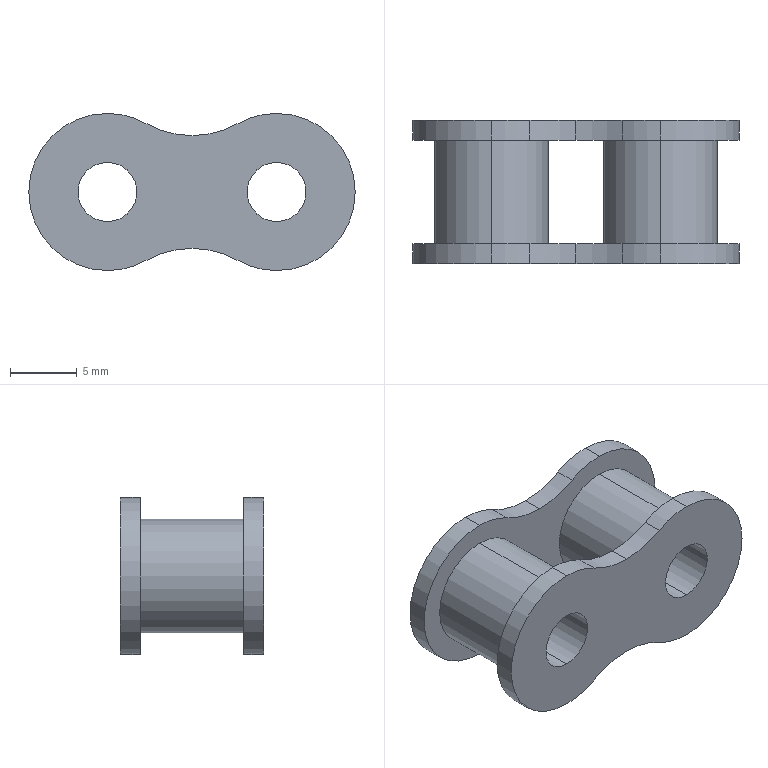Part | SolidWorks | features BaseBody 1 | 1 solid | 30 faces | box 24.5 x 10.75 x 11.8 mm | volume 1261 mm3 | cylinder 26 | plane 4 | commonest cylinder face diameters 11.8 x12 14.097 x6 4.44 x4 8.51 x4
STEP:
#1=CARTESIAN_POINT('',(-429.426,-311.093,-257.788));
#2=VERTEX_POINT('',#1);
#3=CARTESIAN_POINT('',(-429.426,-311.093,-253.348));
#4=VERTEX_POINT('',#3);
#5=CARTESIAN_POINT('',(-429.426,-311.093,-255.568));
#6=DIRECTION('',(0.,1.,0.));
#7=DIRECTION('',(0.,0.,-1.));
#8=AXIS2_PLACEMENT_3D('',#5,#6,#7);
#9=CIRCLE('',#8,2.22);
#10=EDGE_CURVE('',#2,#4,#9,.T.);
#11=ORIENTED_EDGE('',*,*,#10,.T.);
#12=CARTESIAN_POINT('',(-429.426,-321.843,-253.348));
#13=VERTEX_POINT('',#12);
#14=CARTESIAN_POINT('',(-429.426,-312.593,-253.348));
#15=DIRECTION('',(0.,-1.,0.));
#16=VECTOR('',#15,1000.);
#17=LINE('',#14,#16);
#18=EDGE_CURVE('',#4,#13,#17,.T.);
#19=ORIENTED_EDGE('',*,*,#18,.T.);
#20=CARTESIAN_POINT('',(-429.426,-321.843,-257.788));
#21=VERTEX_POINT('',#20);
#22=CARTESIAN_POINT('',(-429.426,-321.843,-255.568));
#23=DIRECTION('',(0.,1.,0.));
#24=DIRECTION('',(-1.,0.,0.));
#25=AXIS2_PLACEMENT_3D('',#22,#23,#24);
#26=CIRCLE('',#25,2.22);
#27=EDGE_CURVE('',#21,#13,#26,.T.);
#28=ORIENTED_EDGE('',*,*,#27,.F.);
#29=CARTESIAN_POINT('',(-429.426,-312.593,-257.788));
#30=DIRECTION('',(0.,-1.,0.));
#31=VECTOR('',#30,1000.);
#32=LINE('',#29,#31);
#33=EDGE_CURVE('',#2,#21,#32,.T.);
#34=ORIENTED_EDGE('',*,*,#33,.F.);
#35=EDGE_LOOP('',(#11,#19,#28,#34));
#36=FACE_OUTER_BOUND('',#35,.T.);
#37=CARTESIAN_POINT('',(-429.426,-312.593,-255.568));
#38=DIRECTION('',(0.,-1.,0.));
#39=DIRECTION('',(0.,0.,-1.));
#40=AXIS2_PLACEMENT_3D('',#37,#38,#39);
#41=CYLINDRICAL_SURFACE('',#40,2.22);
#42=ADVANCED_FACE('',(#36),#41,.F.);
#43=CARTESIAN_POINT('',(-429.426,-312.593,-251.313));
#44=VERTEX_POINT('',#43);
#45=CARTESIAN_POINT('',(-429.426,-312.593,-259.823));
#46=VERTEX_POINT('',#45);
#47=CARTESIAN_POINT('',(-429.426,-312.593,-255.568));
#48=DIRECTION('',(0.,1.,0.));
#49=DIRECTION('',(-1.,0.,0.));
#50=AXIS2_PLACEMENT_3D('',#47,#48,#49);
#51=CIRCLE('',#50,4.255);
#52=EDGE_CURVE('',#44,#46,#51,.T.);
#53=ORIENTED_EDGE('',*,*,#52,.F.);
#54=CARTESIAN_POINT('',(-429.426,-320.343,-251.313));
#55=VERTEX_POINT('',#54);
#56=CARTESIAN_POINT('',(-429.426,-312.593,-251.313));
#57=DIRECTION('',(0.,-1.,0.));
#58=VECTOR('',#57,1000.);
#59=LINE('',#56,#58);
#60=EDGE_CURVE('',#44,#55,#59,.T.);
#61=ORIENTED_EDGE('',*,*,#60,.T.);
#62=CARTESIAN_POINT('',(-429.426,-320.343,-259.823));
#63=VERTEX_POINT('',#62);
#64=CARTESIAN_POINT('',(-429.426,-320.343,-255.568));
#65=DIRECTION('',(0.,1.,0.));
#66=DIRECTION('',(0.,0.,-1.));
#67=AXIS2_PLACEMENT_3D('',#64,#65,#66);
#68=CIRCLE('',#67,4.255);
#69=EDGE_CURVE('',#55,#63,#68,.T.);
#70=ORIENTED_EDGE('',*,*,#69,.T.);
#71=CARTESIAN_POINT('',(-429.426,-312.593,-259.823));
#72=DIRECTION('',(0.,-1.,0.));
#73=VECTOR('',#72,1000.);
#74=LINE('',#71,#73);
#75=EDGE_CURVE('',#46,#63,#74,.T.);
#76=ORIENTED_EDGE('',*,*,#75,.F.);
#77=EDGE_LOOP('',(#53,#61,#70,#76));
#78=FACE_OUTER_BOUND('',#77,.T.);
#79=CARTESIAN_POINT('',(-429.426,-312.593,-255.568));
#80=DIRECTION('',(0.,-1.,0.));
#81=DIRECTION('',(0.,0.,-1.));
#82=AXIS2_PLACEMENT_3D('',#79,#80,#81);
#83=CYLINDRICAL_SURFACE('',#82,4.255);
#84=ADVANCED_FACE('',(#78),#83,.T.);
#85=CARTESIAN_POINT('',(-429.426,-311.093,-249.668));
#86=VERTEX_POINT('',#85);
#87=CARTESIAN_POINT('',(-429.426,-311.093,-261.468));
#88=VERTEX_POINT('',#87);
#89=CARTESIAN_POINT('',(-429.426,-311.093,-255.568));
#90=DIRECTION('',(0.,1.,0.));
#91=DIRECTION('',(-1.,0.,0.));
#92=AXIS2_PLACEMENT_3D('',#89,#90,#91);
#93=CIRCLE('',#92,5.9);
#94=EDGE_CURVE('',#86,#88,#93,.T.);
#95=ORIENTED_EDGE('',*,*,#94,.F.);
#96=CARTESIAN_POINT('',(-429.426,-312.593,-249.668));
#97=VERTEX_POINT('',#96);
#98=CARTESIAN_POINT('',(-429.426,-311.093,-249.668));
#99=DIRECTION('',(0.,-1.,0.));
#100=VECTOR('',#99,1000.);
#101=LINE('',#98,#100);
#102=EDGE_CURVE('',#86,#97,#101,.T.);
#103=ORIENTED_EDGE('',*,*,#102,.T.);
#104=CARTESIAN_POINT('',(-429.426,-312.593,-261.468));
#105=VERTEX_POINT('',#104);
#106=CARTESIAN_POINT('',(-429.426,-312.593,-255.568));
#107=DIRECTION('',(0.,1.,0.));
#108=DIRECTION('',(-1.,0.,0.));
#109=AXIS2_PLACEMENT_3D('',#106,#107,#108);
#110=CIRCLE('',#109,5.9);
#111=EDGE_CURVE('',#97,#105,#110,.T.);
#112=ORIENTED_EDGE('',*,*,#111,.T.);
#113=CARTESIAN_POINT('',(-429.426,-311.093,-261.468));
#114=DIRECTION('',(0.,-1.,0.));
#115=VECTOR('',#114,1000.);
#116=LINE('',#113,#115);
#117=EDGE_CURVE('',#88,#105,#116,.T.);
#118=ORIENTED_EDGE('',*,*,#117,.F.);
#119=EDGE_LOOP('',(#95,#103,#112,#118));
#120=FACE_OUTER_BOUND('',#119,.T.);
#121=CARTESIAN_POINT('',(-429.426,-311.093,-255.568));
#122=DIRECTION('',(0.,-1.,0.));
#123=DIRECTION('',(0.,0.,-1.));
#124=AXIS2_PLACEMENT_3D('',#121,#122,#123);
#125=CYLINDRICAL_SURFACE('',#124,5.9);
#126=ADVANCED_FACE('',(#120),#125,.T.);
#127=CARTESIAN_POINT('',(-432.319,-311.093,-260.71));
#128=VERTEX_POINT('',#127);
#129=CARTESIAN_POINT('',(-429.426,-311.093,-255.568));
#130=DIRECTION('',(0.,1.,0.));
#131=DIRECTION('',(-1.,0.,0.));
#132=AXIS2_PLACEMENT_3D('',#129,#130,#131);
#133=CIRCLE('',#132,5.9);
#134=EDGE_CURVE('',#88,#128,#133,.T.);
#135=ORIENTED_EDGE('',*,*,#134,.F.);
#136=ORIENTED_EDGE('',*,*,#117,.T.);
#137=CARTESIAN_POINT('',(-432.319,-312.593,-260.71));
#138=VERTEX_POINT('',#137);
#139=CARTESIAN_POINT('',(-429.426,-312.593,-255.568));
#140=DIRECTION('',(0.,1.,0.));
#141=DIRECTION('',(-1.,0.,0.));
#142=AXIS2_PLACEMENT_3D('',#139,#140,#141);
#143=CIRCLE('',#142,5.9);
#144=EDGE_CURVE('',#105,#138,#143,.T.);
#145=ORIENTED_EDGE('',*,*,#144,.T.);
#146=CARTESIAN_POINT('',(-432.319,-311.093,-260.71));
#147=DIRECTION('',(0.,-1.,0.));
#148=VECTOR('',#147,1000.);
#149=LINE('',#146,#148);
#150=EDGE_CURVE('',#128,#138,#149,.T.);
#151=ORIENTED_EDGE('',*,*,#150,.F.);
#152=EDGE_LOOP('',(#135,#136,#145,#151));
#153=FACE_OUTER_BOUND('',#152,.T.);
#154=CARTESIAN_POINT('',(-429.426,-311.093,-255.568));
#155=DIRECTION('',(0.,-1.,0.));
#156=DIRECTION('',(0.,0.,-1.));
#157=AXIS2_PLACEMENT_3D('',#154,#155,#156);
#158=CYLINDRICAL_SURFACE('',#157,5.9);
#159=ADVANCED_FACE('',(#153),#158,.T.);
#160=CARTESIAN_POINT('',(-435.776,-311.093,-251.332));
#161=VERTEX_POINT('',#160);
#162=CARTESIAN_POINT('',(-432.319,-311.093,-250.426));
#163=VERTEX_POINT('',#162);
#164=CARTESIAN_POINT('',(-435.776,-311.093,-244.284));
#165=DIRECTION('',(0.,-1.,0.));
#166=DIRECTION('',(-1.,0.,0.));
#167=AXIS2_PLACEMENT_3D('',#164,#165,#166);
#168=CIRCLE('',#167,7.048);
#169=EDGE_CURVE('',#161,#163,#168,.T.);
#170=ORIENTED_EDGE('',*,*,#169,.F.);
#171=CARTESIAN_POINT('',(-435.776,-312.593,-251.332));
#172=VERTEX_POINT('',#171);
#173=CARTESIAN_POINT('',(-435.776,-311.093,-251.332));
#174=DIRECTION('',(0.,-1.,0.));
#175=VECTOR('',#174,1000.);
#176=LINE('',#173,#175);
#177=EDGE_CURVE('',#161,#172,#176,.T.);
#178=ORIENTED_EDGE('',*,*,#177,.T.);
#179=CARTESIAN_POINT('',(-432.319,-312.593,-250.426));
#180=VERTEX_POINT('',#179);
#181=CARTESIAN_POINT('',(-435.776,-312.593,-244.284));
#182=DIRECTION('',(0.,-1.,0.));
#183=DIRECTION('',(-1.,0.,0.));
#184=AXIS2_PLACEMENT_3D('',#181,#182,#183);
#185=CIRCLE('',#184,7.048);
#186=EDGE_CURVE('',#172,#180,#185,.T.);
#187=ORIENTED_EDGE('',*,*,#186,.T.);
#188=CARTESIAN_POINT('',(-432.319,-311.093,-250.426));
#189=DIRECTION('',(0.,-1.,0.));
#190=VECTOR('',#189,1000.);
#191=LINE('',#188,#190);
#192=EDGE_CURVE('',#163,#180,#191,.T.);
#193=ORIENTED_EDGE('',*,*,#192,.F.);
#194=EDGE_LOOP('',(#170,#178,#187,#193));
#195=FACE_OUTER_BOUND('',#194,.T.);
#196=CARTESIAN_POINT('',(-435.776,-311.093,-244.284));
#197=DIRECTION('',(0.,-1.,0.));
#198=DIRECTION('',(0.,0.,-1.));
#199=AXIS2_PLACEMENT_3D('',#196,#197,#198);
#200=CYLINDRICAL_SURFACE('',#199,7.048);
#201=ADVANCED_FACE('',(#195),#200,.F.);
#202=CARTESIAN_POINT('',(-442.126,-311.093,-249.668));
#203=VERTEX_POINT('',#202);
#204=CARTESIAN_POINT('',(-439.232,-311.093,-250.426));
#205=VERTEX_POINT('',#204);
#206=CARTESIAN_POINT('',(-442.126,-311.093,-255.568));
#207=DIRECTION('',(0.,1.,0.));
#208=DIRECTION('',(-1.,0.,0.));
#209=AXIS2_PLACEMENT_3D('',#206,#207,#208);
#210=CIRCLE('',#209,5.9);
#211=EDGE_CURVE('',#203,#205,#210,.T.);
#212=ORIENTED_EDGE('',*,*,#211,.F.);
#213=CARTESIAN_POINT('',(-442.126,-312.593,-249.668));
#214=VERTEX_POINT('',#213);
#215=CARTESIAN_POINT('',(-442.126,-311.093,-249.668));
#216=DIRECTION('',(0.,-1.,0.));
#217=VECTOR('',#216,1000.);
#218=LINE('',#215,#217);
#219=EDGE_CURVE('',#203,#214,#218,.T.);
#220=ORIENTED_EDGE('',*,*,#219,.T.);
#221=CARTESIAN_POINT('',(-439.232,-312.593,-250.426));
#222=VERTEX_POINT('',#221);
#223=CARTESIAN_POINT('',(-442.126,-312.593,-255.568));
#224=DIRECTION('',(0.,1.,0.));
#225=DIRECTION('',(-1.,0.,0.));
#226=AXIS2_PLACEMENT_3D('',#223,#224,#225);
#227=CIRCLE('',#226,5.9);
#228=EDGE_CURVE('',#214,#222,#227,.T.);
#229=ORIENTED_EDGE('',*,*,#228,.T.);
#230=CARTESIAN_POINT('',(-439.232,-311.093,-250.426));
#231=DIRECTION('',(0.,-1.,0.));
#232=VECTOR('',#231,1000.);
#233=LINE('',#230,#232);
#234=EDGE_CURVE('',#205,#222,#233,.T.);
#235=ORIENTED_EDGE('',*,*,#234,.F.);
#236=EDGE_LOOP('',(#212,#220,#229,#235));
#237=FACE_OUTER_BOUND('',#236,.T.);
#238=CARTESIAN_POINT('',(-442.126,-311.093,-255.568));
#239=DIRECTION('',(0.,-1.,0.));
#240=DIRECTION('',(0.,0.,-1.));
#241=AXIS2_PLACEMENT_3D('',#238,#239,#240);
#242=CYLINDRICAL_SURFACE('',#241,5.9);
#243=ADVANCED_FACE('',(#237),#242,.T.);
#244=ORIENTED_EDGE('',*,*,#219,.F.);
#245=CARTESIAN_POINT('',(-442.126,-311.093,-261.468));
#246=VERTEX_POINT('',#245);
#247=CARTESIAN_POINT('',(-442.126,-311.093,-255.568));
#248=DIRECTION('',(0.,1.,0.));
#249=DIRECTION('',(-1.,0.,0.));
#250=AXIS2_PLACEMENT_3D('',#247,#248,#249);
#251=CIRCLE('',#250,5.9);
#252=EDGE_CURVE('',#246,#203,#251,.T.);
#253=ORIENTED_EDGE('',*,*,#252,.F.);
#254=CARTESIAN_POINT('',(-442.126,-312.593,-261.468));
#255=VERTEX_POINT('',#254);
#256=CARTESIAN_POINT('',(-442.126,-311.093,-261.468));
#257=DIRECTION('',(0.,-1.,0.));
#258=VECTOR('',#257,1000.);
#259=LINE('',#256,#258);
#260=EDGE_CURVE('',#246,#255,#259,.T.);
#261=ORIENTED_EDGE('',*,*,#260,.T.);
#262=CARTESIAN_POINT('',(-442.126,-312.593,-255.568));
#263=DIRECTION('',(0.,1.,0.));
#264=DIRECTION('',(-1.,0.,0.));
#265=AXIS2_PLACEMENT_3D('',#262,#263,#264);
#266=CIRCLE('',#265,5.9);
#267=EDGE_CURVE('',#255,#214,#266,.T.);
#268=ORIENTED_EDGE('',*,*,#267,.T.);
#269=EDGE_LOOP('',(#244,#253,#261,#268));
#270=FACE_OUTER_BOUND('',#269,.T.);
#271=CARTESIAN_POINT('',(-442.126,-311.093,-255.568));
#272=DIRECTION('',(0.,-1.,0.));
#273=DIRECTION('',(0.,0.,-1.));
#274=AXIS2_PLACEMENT_3D('',#271,#272,#273);
#275=CYLINDRICAL_SURFACE('',#274,5.9);
#276=ADVANCED_FACE('',(#270),#275,.T.);
#277=CARTESIAN_POINT('',(-429.426,-320.343,-249.668));
#278=VERTEX_POINT('',#277);
#279=CARTESIAN_POINT('',(-429.426,-320.343,-261.468));
#280=VERTEX_POINT('',#279);
#281=CARTESIAN_POINT('',(-429.426,-320.343,-255.568));
#282=DIRECTION('',(0.,1.,0.));
#283=DIRECTION('',(-1.,0.,0.));
#284=AXIS2_PLACEMENT_3D('',#281,#282,#283);
#285=CIRCLE('',#284,5.9);
#286=EDGE_CURVE('',#278,#280,#285,.T.);
#287=ORIENTED_EDGE('',*,*,#286,.F.);
#288=CARTESIAN_POINT('',(-429.426,-321.843,-249.668));
#289=VERTEX_POINT('',#288);
#290=CARTESIAN_POINT('',(-429.426,-320.343,-249.668));
#291=DIRECTION('',(0.,-1.,0.));
#292=VECTOR('',#291,1000.);
#293=LINE('',#290,#292);
#294=EDGE_CURVE('',#278,#289,#293,.T.);
#295=ORIENTED_EDGE('',*,*,#294,.T.);
#296=CARTESIAN_POINT('',(-429.426,-321.843,-261.468));
#297=VERTEX_POINT('',#296);
#298=CARTESIAN_POINT('',(-429.426,-321.843,-255.568));
#299=DIRECTION('',(0.,1.,0.));
#300=DIRECTION('',(-1.,0.,0.));
#301=AXIS2_PLACEMENT_3D('',#298,#299,#300);
#302=CIRCLE('',#301,5.9);
#303=EDGE_CURVE('',#289,#297,#302,.T.);
#304=ORIENTED_EDGE('',*,*,#303,.T.);
#305=CARTESIAN_POINT('',(-429.426,-320.343,-261.468));
#306=DIRECTION('',(0.,-1.,0.));
#307=VECTOR('',#306,1000.);
#308=LINE('',#305,#307);
#309=EDGE_CURVE('',#280,#297,#308,.T.);
#310=ORIENTED_EDGE('',*,*,#309,.F.);
#311=EDGE_LOOP('',(#287,#295,#304,#310));
#312=FACE_OUTER_BOUND('',#311,.T.);
#313=CARTESIAN_POINT('',(-429.426,-320.343,-255.568));
#314=DIRECTION('',(0.,-1.,0.));
#315=DIRECTION('',(0.,0.,-1.));
#316=AXIS2_PLACEMENT_3D('',#313,#314,#315);
#317=CYLINDRICAL_SURFACE('',#316,5.9);
#318=ADVANCED_FACE('',(#312),#317,.T.);
#319=CARTESIAN_POINT('',(-432.319,-320.343,-260.71));
#320=VERTEX_POINT('',#319);
#321=CARTESIAN_POINT('',(-429.426,-320.343,-255.568));
#322=DIRECTION('',(0.,1.,0.));
#323=DIRECTION('',(-1.,0.,0.));
#324=AXIS2_PLACEMENT_3D('',#321,#322,#323);
#325=CIRCLE('',#324,5.9);
#326=EDGE_CURVE('',#280,#320,#325,.T.);
#327=ORIENTED_EDGE('',*,*,#326,.F.);
#328=ORIENTED_EDGE('',*,*,#309,.T.);
#329=CARTESIAN_POINT('',(-432.319,-321.843,-260.71));
#330=VERTEX_POINT('',#329);
#331=CARTESIAN_POINT('',(-429.426,-321.843,-255.568));
#332=DIRECTION('',(0.,1.,0.));
#333=DIRECTION('',(-1.,0.,0.));
#334=AXIS2_PLACEMENT_3D('',#331,#332,#333);
#335=CIRCLE('',#334,5.9);
#336=EDGE_CURVE('',#297,#330,#335,.T.);
#337=ORIENTED_EDGE('',*,*,#336,.T.);
#338=CARTESIAN_POINT('',(-432.319,-320.343,-260.71));
#339=DIRECTION('',(0.,-1.,0.));
#340=VECTOR('',#339,1000.);
#341=LINE('',#338,#340);
#342=EDGE_CURVE('',#320,#330,#341,.T.);
#343=ORIENTED_EDGE('',*,*,#342,.F.);
#344=EDGE_LOOP('',(#327,#328,#337,#343));
#345=FACE_OUTER_BOUND('',#344,.T.);
#346=CARTESIAN_POINT('',(-429.426,-320.343,-255.568));
#347=DIRECTION('',(0.,-1.,0.));
#348=DIRECTION('',(0.,0.,-1.));
#349=AXIS2_PLACEMENT_3D('',#346,#347,#348);
#350=CYLINDRICAL_SURFACE('',#349,5.9);
#351=ADVANCED_FACE('',(#345),#350,.T.);
#352=CARTESIAN_POINT('',(-435.776,-320.343,-251.332));
#353=VERTEX_POINT('',#352);
#354=CARTESIAN_POINT('',(-432.319,-320.343,-250.426));
#355=VERTEX_POINT('',#354);
#356=CARTESIAN_POINT('',(-435.776,-320.343,-244.284));
#357=DIRECTION('',(0.,-1.,0.));
#358=DIRECTION('',(-1.,0.,0.));
#359=AXIS2_PLACEMENT_3D('',#356,#357,#358);
#360=CIRCLE('',#359,7.048);
#361=EDGE_CURVE('',#353,#355,#360,.T.);
#362=ORIENTED_EDGE('',*,*,#361,.F.);
#363=CARTESIAN_POINT('',(-435.776,-321.843,-251.332));
#364=VERTEX_POINT('',#363);
#365=CARTESIAN_POINT('',(-435.776,-320.343,-251.332));
#366=DIRECTION('',(0.,-1.,0.));
#367=VECTOR('',#366,1000.);
#368=LINE('',#365,#367);
#369=EDGE_CURVE('',#353,#364,#368,.T.);
#370=ORIENTED_EDGE('',*,*,#369,.T.);
#371=CARTESIAN_POINT('',(-432.319,-321.843,-250.426));
#372=VERTEX_POINT('',#371);
#373=CARTESIAN_POINT('',(-435.776,-321.843,-244.284));
#374=DIRECTION('',(0.,-1.,0.));
#375=DIRECTION('',(-1.,0.,0.));
#376=AXIS2_PLACEMENT_3D('',#373,#374,#375);
#377=CIRCLE('',#376,7.048);
#378=EDGE_CURVE('',#364,#372,#377,.T.);
#379=ORIENTED_EDGE('',*,*,#378,.T.);
#380=CARTESIAN_POINT('',(-432.319,-320.343,-250.426));
#381=DIRECTION('',(0.,-1.,0.));
#382=VECTOR('',#381,1000.);
#383=LINE('',#380,#382);
#384=EDGE_CURVE('',#355,#372,#383,.T.);
#385=ORIENTED_EDGE('',*,*,#384,.F.);
#386=EDGE_LOOP('',(#362,#370,#379,#385));
#387=FACE_OUTER_BOUND('',#386,.T.);
#388=CARTESIAN_POINT('',(-435.776,-320.343,-244.284));
#389=DIRECTION('',(0.,-1.,0.));
#390=DIRECTION('',(0.,0.,-1.));
#391=AXIS2_PLACEMENT_3D('',#388,#389,#390);
#392=CYLINDRICAL_SURFACE('',#391,7.048);
#393=ADVANCED_FACE('',(#387),#392,.F.);
#394=CARTESIAN_POINT('',(-442.126,-320.343,-249.668));
#395=VERTEX_POINT('',#394);
#396=CARTESIAN_POINT('',(-439.232,-320.343,-250.426));
#397=VERTEX_POINT('',#396);
#398=CARTESIAN_POINT('',(-442.126,-320.343,-255.568));
#399=DIRECTION('',(0.,1.,0.));
#400=DIRECTION('',(-1.,0.,0.));
#401=AXIS2_PLACEMENT_3D('',#398,#399,#400);
#402=CIRCLE('',#401,5.9);
#403=EDGE_CURVE('',#395,#397,#402,.T.);
#404=ORIENTED_EDGE('',*,*,#403,.F.);
#405=CARTESIAN_POINT('',(-442.126,-321.843,-249.668));
#406=VERTEX_POINT('',#405);
#407=CARTESIAN_POINT('',(-442.126,-320.343,-249.668));
#408=DIRECTION('',(0.,-1.,0.));
#409=VECTOR('',#408,1000.);
#410=LINE('',#407,#409);
#411=EDGE_CURVE('',#395,#406,#410,.T.);
#412=ORIENTED_EDGE('',*,*,#411,.T.);
#413=CARTESIAN_POINT('',(-439.232,-321.843,-250.426));
#414=VERTEX_POINT('',#413);
#415=CARTESIAN_POINT('',(-442.126,-321.843,-255.568));
#416=DIRECTION('',(0.,1.,0.));
#417=DIRECTION('',(-1.,0.,0.));
#418=AXIS2_PLACEMENT_3D('',#415,#416,#417);
#419=CIRCLE('',#418,5.9);
#420=EDGE_CURVE('',#406,#414,#419,.T.);
#421=ORIENTED_EDGE('',*,*,#420,.T.);
#422=CARTESIAN_POINT('',(-439.232,-320.343,-250.426));
#423=DIRECTION('',(0.,-1.,0.));
#424=VECTOR('',#423,1000.);
#425=LINE('',#422,#424);
#426=EDGE_CURVE('',#397,#414,#425,.T.);
#427=ORIENTED_EDGE('',*,*,#426,.F.);
#428=EDGE_LOOP('',(#404,#412,#421,#427));
#429=FACE_OUTER_BOUND('',#428,.T.);
#430=CARTESIAN_POINT('',(-442.126,-320.343,-255.568));
#431=DIRECTION('',(0.,-1.,0.));
#432=DIRECTION('',(0.,0.,-1.));
#433=AXIS2_PLACEMENT_3D('',#430,#431,#432);
#434=CYLINDRICAL_SURFACE('',#433,5.9);
#435=ADVANCED_FACE('',(#429),#434,.T.);
#436=ORIENTED_EDGE('',*,*,#411,.F.);
#437=CARTESIAN_POINT('',(-442.126,-320.343,-261.468));
#438=VERTEX_POINT('',#437);
#439=CARTESIAN_POINT('',(-442.126,-320.343,-255.568));
#440=DIRECTION('',(0.,1.,0.));
#441=DIRECTION('',(-1.,0.,0.));
#442=AXIS2_PLACEMENT_3D('',#439,#440,#441);
#443=CIRCLE('',#442,5.9);
#444=EDGE_CURVE('',#438,#395,#443,.T.);
#445=ORIENTED_EDGE('',*,*,#444,.F.);
#446=CARTESIAN_POINT('',(-442.126,-321.843,-261.468));
#447=VERTEX_POINT('',#446);
#448=CARTESIAN_POINT('',(-442.126,-320.343,-261.468));
#449=DIRECTION('',(0.,-1.,0.));
#450=VECTOR('',#449,1000.);
#451=LINE('',#448,#450);
#452=EDGE_CURVE('',#438,#447,#451,.T.);
#453=ORIENTED_EDGE('',*,*,#452,.T.);
#454=CARTESIAN_POINT('',(-442.126,-321.843,-255.568));
#455=DIRECTION('',(0.,1.,0.));
#456=DIRECTION('',(-1.,0.,0.));
#457=AXIS2_PLACEMENT_3D('',#454,#455,#456);
#458=CIRCLE('',#457,5.9);
#459=EDGE_CURVE('',#447,#406,#458,.T.);
#460=ORIENTED_EDGE('',*,*,#459,.T.);
#461=EDGE_LOOP('',(#436,#445,#453,#460));
#462=FACE_OUTER_BOUND('',#461,.T.);
#463=CARTESIAN_POINT('',(-442.126,-320.343,-255.568));
#464=DIRECTION('',(0.,-1.,0.));
#465=DIRECTION('',(0.,0.,-1.));
#466=AXIS2_PLACEMENT_3D('',#463,#464,#465);
#467=CYLINDRICAL_SURFACE('',#466,5.9);
#468=ADVANCED_FACE('',(#462),#467,.T.);
#469=CARTESIAN_POINT('',(-442.126,-311.093,-257.788));
#470=VERTEX_POINT('',#469);
#471=CARTESIAN_POINT('',(-442.126,-311.093,-253.348));
#472=VERTEX_POINT('',#471);
#473=CARTESIAN_POINT('',(-442.126,-311.093,-255.568));
#474=DIRECTION('',(0.,1.,0.));
#475=DIRECTION('',(0.,0.,-1.));
#476=AXIS2_PLACEMENT_3D('',#473,#474,#475);
#477=CIRCLE('',#476,2.22);
#478=EDGE_CURVE('',#470,#472,#477,.T.);
#479=ORIENTED_EDGE('',*,*,#478,.T.);
#480=CARTESIAN_POINT('',(-442.126,-321.843,-253.348));
#481=VERTEX_POINT('',#480);
#482=CARTESIAN_POINT('',(-442.126,-312.593,-253.348));
#483=DIRECTION('',(0.,-1.,0.));
#484=VECTOR('',#483,1000.);
#485=LINE('',#482,#484);
#486=EDGE_CURVE('',#472,#481,#485,.T.);
#487=ORIENTED_EDGE('',*,*,#486,.T.);
#488=CARTESIAN_POINT('',(-442.126,-321.843,-257.788));
#489=VERTEX_POINT('',#488);
#490=CARTESIAN_POINT('',(-442.126,-321.843,-255.568));
#491=DIRECTION('',(0.,1.,0.));
#492=DIRECTION('',(-1.,0.,0.));
#493=AXIS2_PLACEMENT_3D('',#490,#491,#492);
#494=CIRCLE('',#493,2.22);
#495=EDGE_CURVE('',#489,#481,#494,.T.);
#496=ORIENTED_EDGE('',*,*,#495,.F.);
#497=CARTESIAN_POINT('',(-442.126,-312.593,-257.788));
#498=DIRECTION('',(0.,-1.,0.));
#499=VECTOR('',#498,1000.);
#500=LINE('',#497,#499);
#501=EDGE_CURVE('',#470,#489,#500,.T.);
#502=ORIENTED_EDGE('',*,*,#501,.F.);
#503=EDGE_LOOP('',(#479,#487,#496,#502));
#504=FACE_OUTER_BOUND('',#503,.T.);
#505=CARTESIAN_POINT('',(-442.126,-312.593,-255.568));
#506=DIRECTION('',(0.,-1.,0.));
#507=DIRECTION('',(0.,0.,-1.));
#508=AXIS2_PLACEMENT_3D('',#505,#506,#507);
#509=CYLINDRICAL_SURFACE('',#508,2.22);
#510=ADVANCED_FACE('',(#504),#509,.F.);
#511=CARTESIAN_POINT('',(-442.126,-312.593,-259.823));
#512=VERTEX_POINT('',#511);
#513=CARTESIAN_POINT('',(-442.126,-312.593,-251.313));
#514=VERTEX_POINT('',#513);
#515=CARTESIAN_POINT('',(-442.126,-312.593,-255.568));
#516=DIRECTION('',(0.,-1.,0.));
#517=DIRECTION('',(0.,0.,-1.));
#518=AXIS2_PLACEMENT_3D('',#515,#516,#517);
#519=CIRCLE('',#518,4.255);
#520=EDGE_CURVE('',#512,#514,#519,.T.);
#521=ORIENTED_EDGE('',*,*,#520,.T.);
#522=CARTESIAN_POINT('',(-442.126,-320.343,-251.313));
#523=VERTEX_POINT('',#522);
#524=CARTESIAN_POINT('',(-442.126,-312.593,-251.313));
#525=DIRECTION('',(0.,-1.,0.));
#526=VECTOR('',#525,1000.);
#527=LINE('',#524,#526);
#528=EDGE_CURVE('',#514,#523,#527,.T.);
#529=ORIENTED_EDGE('',*,*,#528,.T.);
#530=CARTESIAN_POINT('',(-442.126,-320.343,-259.823));
#531=VERTEX_POINT('',#530);
#532=CARTESIAN_POINT('',(-442.126,-320.343,-255.568));
#533=DIRECTION('',(0.,1.,0.));
#534=DIRECTION('',(-1.,0.,0.));
#535=AXIS2_PLACEMENT_3D('',#532,#533,#534);
#536=CIRCLE('',#535,4.255);
#537=EDGE_CURVE('',#523,#531,#536,.T.);
#538=ORIENTED_EDGE('',*,*,#537,.T.);
#539=CARTESIAN_POINT('',(-442.126,-312.593,-259.823));
#540=DIRECTION('',(0.,-1.,0.));
#541=VECTOR('',#540,1000.);
#542=LINE('',#539,#541);
#543=EDGE_CURVE('',#512,#531,#542,.T.);
#544=ORIENTED_EDGE('',*,*,#543,.F.);
#545=EDGE_LOOP('',(#521,#529,#538,#544));
#546=FACE_OUTER_BOUND('',#545,.T.);
#547=CARTESIAN_POINT('',(-442.126,-312.593,-255.568));
#548=DIRECTION('',(0.,-1.,0.));
#549=DIRECTION('',(0.,0.,-1.));
#550=AXIS2_PLACEMENT_3D('',#547,#548,#549);
#551=CYLINDRICAL_SURFACE('',#550,4.255);
#552=ADVANCED_FACE('',(#546),#551,.T.);
#553=ORIENTED_EDGE('',*,*,#528,.F.);
#554=CARTESIAN_POINT('',(-442.126,-312.593,-255.568));
#555=DIRECTION('',(0.,-1.,0.));
#556=DIRECTION('',(0.,0.,-1.));
#557=AXIS2_PLACEMENT_3D('',#554,#555,#556);
#558=CIRCLE('',#557,4.255);
#559=EDGE_CURVE('',#514,#512,#558,.T.);
#560=ORIENTED_EDGE('',*,*,#559,.T.);
#561=ORIENTED_EDGE('',*,*,#543,.T.);
#562=CARTESIAN_POINT('',(-442.126,-320.343,-255.568));
#563=DIRECTION('',(0.,1.,0.));
#564=DIRECTION('',(-1.,0.,0.));
#565=AXIS2_PLACEMENT_3D('',#562,#563,#564);
#566=CIRCLE('',#565,4.255);
#567=EDGE_CURVE('',#531,#523,#566,.T.);
#568=ORIENTED_EDGE('',*,*,#567,.T.);
#569=EDGE_LOOP('',(#553,#560,#561,#568));
#570=FACE_OUTER_BOUND('',#569,.T.);
#571=CARTESIAN_POINT('',(-442.126,-312.593,-255.568));
#572=DIRECTION('',(0.,-1.,0.));
#573=DIRECTION('',(0.,0.,-1.));
#574=AXIS2_PLACEMENT_3D('',#571,#572,#573);
#575=CYLINDRICAL_SURFACE('',#574,4.255);
#576=ADVANCED_FACE('',(#570),#575,.T.);
#577=ORIENTED_EDGE('',*,*,#486,.F.);
#578=CARTESIAN_POINT('',(-442.126,-311.093,-255.568));
#579=DIRECTION('',(0.,1.,0.));
#580=DIRECTION('',(0.,0.,-1.));
#581=AXIS2_PLACEMENT_3D('',#578,#579,#580);
#582=CIRCLE('',#581,2.22);
#583=EDGE_CURVE('',#472,#470,#582,.T.);
#584=ORIENTED_EDGE('',*,*,#583,.T.);
#585=ORIENTED_EDGE('',*,*,#501,.T.);
#586=CARTESIAN_POINT('',(-442.126,-321.843,-255.568));
#587=DIRECTION('',(0.,1.,0.));
#588=DIRECTION('',(-1.,0.,0.));
#589=AXIS2_PLACEMENT_3D('',#586,#587,#588);
#590=CIRCLE('',#589,2.22);
#591=EDGE_CURVE('',#481,#489,#590,.T.);
#592=ORIENTED_EDGE('',*,*,#591,.F.);
#593=EDGE_LOOP('',(#577,#584,#585,#592));
#594=FACE_OUTER_BOUND('',#593,.T.);
#595=CARTESIAN_POINT('',(-442.126,-312.593,-255.568));
#596=DIRECTION('',(0.,-1.,0.));
#597=DIRECTION('',(0.,0.,-1.));
#598=AXIS2_PLACEMENT_3D('',#595,#596,#597);
#599=CYLINDRICAL_SURFACE('',#598,2.22);
#600=ADVANCED_FACE('',(#594),#599,.F.);
#601=ORIENTED_EDGE('',*,*,#478,.F.);
#602=ORIENTED_EDGE('',*,*,#583,.F.);
#603=EDGE_LOOP('',(#601,#602));
#604=FACE_BOUND('',#603,.T.);
#605=CARTESIAN_POINT('',(-439.232,-311.093,-260.71));
#606=VERTEX_POINT('',#605);
#607=CARTESIAN_POINT('',(-442.126,-311.093,-255.568));
#608=DIRECTION('',(0.,1.,0.));
#609=DIRECTION('',(-1.,0.,0.));
#610=AXIS2_PLACEMENT_3D('',#607,#608,#609);
#611=CIRCLE('',#610,5.9);
#612=EDGE_CURVE('',#606,#246,#611,.T.);
#613=ORIENTED_EDGE('',*,*,#612,.T.);
#614=ORIENTED_EDGE('',*,*,#252,.T.);
#615=ORIENTED_EDGE('',*,*,#211,.T.);
#616=CARTESIAN_POINT('',(-435.776,-311.093,-244.284));
#617=DIRECTION('',(0.,-1.,0.));
#618=DIRECTION('',(-1.,0.,0.));
#619=AXIS2_PLACEMENT_3D('',#616,#617,#618);
#620=CIRCLE('',#619,7.048);
#621=EDGE_CURVE('',#205,#161,#620,.T.);
#622=ORIENTED_EDGE('',*,*,#621,.T.);
#623=ORIENTED_EDGE('',*,*,#169,.T.);
#624=CARTESIAN_POINT('',(-429.426,-311.093,-255.568));
#625=DIRECTION('',(0.,1.,0.));
#626=DIRECTION('',(-1.,0.,0.));
#627=AXIS2_PLACEMENT_3D('',#624,#625,#626);
#628=CIRCLE('',#627,5.9);
#629=EDGE_CURVE('',#163,#86,#628,.T.);
#630=ORIENTED_EDGE('',*,*,#629,.T.);
#631=ORIENTED_EDGE('',*,*,#94,.T.);
#632=ORIENTED_EDGE('',*,*,#134,.T.);
#633=CARTESIAN_POINT('',(-435.776,-311.093,-266.853));
#634=DIRECTION('',(0.,-1.,0.));
#635=DIRECTION('',(-1.,0.,0.));
#636=AXIS2_PLACEMENT_3D('',#633,#634,#635);
#637=CIRCLE('',#636,7.048);
#638=EDGE_CURVE('',#128,#606,#637,.T.);
#639=ORIENTED_EDGE('',*,*,#638,.T.);
#640=EDGE_LOOP('',(#613,#614,#615,#622,#623,#630,#631,#632,#639));
#641=FACE_OUTER_BOUND('',#640,.T.);
#642=ORIENTED_EDGE('',*,*,#10,.F.);
#643=CARTESIAN_POINT('',(-429.426,-311.093,-255.568));
#644=DIRECTION('',(0.,1.,0.));
#645=DIRECTION('',(0.,0.,-1.));
#646=AXIS2_PLACEMENT_3D('',#643,#644,#645);
#647=CIRCLE('',#646,2.22);
#648=EDGE_CURVE('',#4,#2,#647,.T.);
#649=ORIENTED_EDGE('',*,*,#648,.F.);
#650=EDGE_LOOP('',(#642,#649));
#651=FACE_BOUND('',#650,.T.);
#652=CARTESIAN_POINT('',(-438.951,-311.093,-249.926));
#653=DIRECTION('',(0.,-1.,0.));
#654=DIRECTION('',(0.,0.,-1.));
#655=AXIS2_PLACEMENT_3D('',#652,#653,#654);
#656=PLANE('',#655);
#657=ADVANCED_FACE('',(#604,#641,#651),#656,.F.);
#658=ORIENTED_EDGE('',*,*,#495,.T.);
#659=ORIENTED_EDGE('',*,*,#591,.T.);
#660=EDGE_LOOP('',(#658,#659));
#661=FACE_BOUND('',#660,.T.);
#662=CARTESIAN_POINT('',(-439.232,-321.843,-260.71));
#663=VERTEX_POINT('',#662);
#664=CARTESIAN_POINT('',(-442.126,-321.843,-255.568));
#665=DIRECTION('',(0.,1.,0.));
#666=DIRECTION('',(-1.,0.,0.));
#667=AXIS2_PLACEMENT_3D('',#664,#665,#666);
#668=CIRCLE('',#667,5.9);
#669=EDGE_CURVE('',#663,#447,#668,.T.);
#670=ORIENTED_EDGE('',*,*,#669,.F.);
#671=CARTESIAN_POINT('',(-435.776,-321.843,-266.853));
#672=DIRECTION('',(0.,-1.,0.));
#673=DIRECTION('',(-1.,0.,0.));
#674=AXIS2_PLACEMENT_3D('',#671,#672,#673);
#675=CIRCLE('',#674,7.048);
#676=EDGE_CURVE('',#330,#663,#675,.T.);
#677=ORIENTED_EDGE('',*,*,#676,.F.);
#678=ORIENTED_EDGE('',*,*,#336,.F.);
#679=ORIENTED_EDGE('',*,*,#303,.F.);
#680=CARTESIAN_POINT('',(-429.426,-321.843,-255.568));
#681=DIRECTION('',(0.,1.,0.));
#682=DIRECTION('',(-1.,0.,0.));
#683=AXIS2_PLACEMENT_3D('',#680,#681,#682);
#684=CIRCLE('',#683,5.9);
#685=EDGE_CURVE('',#372,#289,#684,.T.);
#686=ORIENTED_EDGE('',*,*,#685,.F.);
#687=ORIENTED_EDGE('',*,*,#378,.F.);
#688=CARTESIAN_POINT('',(-435.776,-321.843,-244.284));
#689=DIRECTION('',(0.,-1.,0.));
#690=DIRECTION('',(-1.,0.,0.));
#691=AXIS2_PLACEMENT_3D('',#688,#689,#690);
#692=CIRCLE('',#691,7.048);
#693=EDGE_CURVE('',#414,#364,#692,.T.);
#694=ORIENTED_EDGE('',*,*,#693,.F.);
#695=ORIENTED_EDGE('',*,*,#420,.F.);
#696=ORIENTED_EDGE('',*,*,#459,.F.);
#697=EDGE_LOOP('',(#670,#677,#678,#679,#686,#687,#694,#695,#696));
#698=FACE_OUTER_BOUND('',#697,.T.);
#699=ORIENTED_EDGE('',*,*,#27,.T.);
#700=CARTESIAN_POINT('',(-429.426,-321.843,-255.568));
#701=DIRECTION('',(0.,1.,0.));
#702=DIRECTION('',(-1.,0.,0.));
#703=AXIS2_PLACEMENT_3D('',#700,#701,#702);
#704=CIRCLE('',#703,2.22);
#705=EDGE_CURVE('',#13,#21,#704,.T.);
#706=ORIENTED_EDGE('',*,*,#705,.T.);
#707=EDGE_LOOP('',(#699,#706));
#708=FACE_BOUND('',#707,.T.);
#709=CARTESIAN_POINT('',(-442.126,-321.843,-255.568));
#710=DIRECTION('',(0.,-1.,0.));
#711=DIRECTION('',(0.,0.,-1.));
#712=AXIS2_PLACEMENT_3D('',#709,#710,#711);
#713=PLANE('',#712);
#714=ADVANCED_FACE('',(#661,#698,#708),#713,.T.);
#715=ORIENTED_EDGE('',*,*,#452,.F.);
#716=CARTESIAN_POINT('',(-439.232,-320.343,-260.71));
#717=VERTEX_POINT('',#716);
#718=CARTESIAN_POINT('',(-442.126,-320.343,-255.568));
#719=DIRECTION('',(0.,1.,0.));
#720=DIRECTION('',(-1.,0.,0.));
#721=AXIS2_PLACEMENT_3D('',#718,#719,#720);
#722=CIRCLE('',#721,5.9);
#723=EDGE_CURVE('',#717,#438,#722,.T.);
#724=ORIENTED_EDGE('',*,*,#723,.F.);
#725=CARTESIAN_POINT('',(-439.232,-320.343,-260.71));
#726=DIRECTION('',(0.,-1.,0.));
#727=VECTOR('',#726,1000.);
#728=LINE('',#725,#727);
#729=EDGE_CURVE('',#717,#663,#728,.T.);
#730=ORIENTED_EDGE('',*,*,#729,.T.);
#731=ORIENTED_EDGE('',*,*,#669,.T.);
#732=EDGE_LOOP('',(#715,#724,#730,#731));
#733=FACE_OUTER_BOUND('',#732,.T.);
#734=CARTESIAN_POINT('',(-442.126,-320.343,-255.568));
#735=DIRECTION('',(0.,-1.,0.));
#736=DIRECTION('',(0.,0.,-1.));
#737=AXIS2_PLACEMENT_3D('',#734,#735,#736);
#738=CYLINDRICAL_SURFACE('',#737,5.9);
#739=ADVANCED_FACE('',(#733),#738,.T.);
#740=ORIENTED_EDGE('',*,*,#369,.F.);
#741=CARTESIAN_POINT('',(-435.776,-320.343,-244.284));
#742=DIRECTION('',(0.,-1.,0.));
#743=DIRECTION('',(-1.,0.,0.));
#744=AXIS2_PLACEMENT_3D('',#741,#742,#743);
#745=CIRCLE('',#744,7.048);
#746=EDGE_CURVE('',#397,#353,#745,.T.);
#747=ORIENTED_EDGE('',*,*,#746,.F.);
#748=ORIENTED_EDGE('',*,*,#426,.T.);
#749=ORIENTED_EDGE('',*,*,#693,.T.);
#750=EDGE_LOOP('',(#740,#747,#748,#749));
#751=FACE_OUTER_BOUND('',#750,.T.);
#752=CARTESIAN_POINT('',(-435.776,-320.343,-244.284));
#753=DIRECTION('',(0.,-1.,0.));
#754=DIRECTION('',(0.,0.,-1.));
#755=AXIS2_PLACEMENT_3D('',#752,#753,#754);
#756=CYLINDRICAL_SURFACE('',#755,7.048);
#757=ADVANCED_FACE('',(#751),#756,.F.);
#758=ORIENTED_EDGE('',*,*,#294,.F.);
#759=CARTESIAN_POINT('',(-429.426,-320.343,-255.568));
#760=DIRECTION('',(0.,1.,0.));
#761=DIRECTION('',(-1.,0.,0.));
#762=AXIS2_PLACEMENT_3D('',#759,#760,#761);
#763=CIRCLE('',#762,5.9);
#764=EDGE_CURVE('',#355,#278,#763,.T.);
#765=ORIENTED_EDGE('',*,*,#764,.F.);
#766=ORIENTED_EDGE('',*,*,#384,.T.);
#767=ORIENTED_EDGE('',*,*,#685,.T.);
#768=EDGE_LOOP('',(#758,#765,#766,#767));
#769=FACE_OUTER_BOUND('',#768,.T.);
#770=CARTESIAN_POINT('',(-429.426,-320.343,-255.568));
#771=DIRECTION('',(0.,-1.,0.));
#772=DIRECTION('',(0.,0.,-1.));
#773=AXIS2_PLACEMENT_3D('',#770,#771,#772);
#774=CYLINDRICAL_SURFACE('',#773,5.9);
#775=ADVANCED_FACE('',(#769),#774,.T.);
#776=ORIENTED_EDGE('',*,*,#676,.T.);
#777=ORIENTED_EDGE('',*,*,#729,.F.);
#778=CARTESIAN_POINT('',(-435.776,-320.343,-266.853));
#779=DIRECTION('',(0.,-1.,0.));
#780=DIRECTION('',(-1.,0.,0.));
#781=AXIS2_PLACEMENT_3D('',#778,#779,#780);
#782=CIRCLE('',#781,7.048);
#783=EDGE_CURVE('',#320,#717,#782,.T.);
#784=ORIENTED_EDGE('',*,*,#783,.F.);
#785=ORIENTED_EDGE('',*,*,#342,.T.);
#786=EDGE_LOOP('',(#776,#777,#784,#785));
#787=FACE_OUTER_BOUND('',#786,.T.);
#788=CARTESIAN_POINT('',(-435.776,-320.343,-266.853));
#789=DIRECTION('',(0.,-1.,0.));
#790=DIRECTION('',(0.,0.,-1.));
#791=AXIS2_PLACEMENT_3D('',#788,#789,#790);
#792=CYLINDRICAL_SURFACE('',#791,7.048);
#793=ADVANCED_FACE('',(#787),#792,.F.);
#794=ORIENTED_EDGE('',*,*,#723,.T.);
#795=ORIENTED_EDGE('',*,*,#444,.T.);
#796=ORIENTED_EDGE('',*,*,#403,.T.);
#797=ORIENTED_EDGE('',*,*,#746,.T.);
#798=ORIENTED_EDGE('',*,*,#361,.T.);
#799=ORIENTED_EDGE('',*,*,#764,.T.);
#800=ORIENTED_EDGE('',*,*,#286,.T.);
#801=ORIENTED_EDGE('',*,*,#326,.T.);
#802=ORIENTED_EDGE('',*,*,#783,.T.);
#803=EDGE_LOOP('',(#794,#795,#796,#797,#798,#799,#800,#801,#802));
#804=FACE_OUTER_BOUND('',#803,.T.);
#805=CARTESIAN_POINT('',(-429.426,-320.343,-255.568));
#806=DIRECTION('',(0.,1.,0.));
#807=DIRECTION('',(0.,0.,-1.));
#808=AXIS2_PLACEMENT_3D('',#805,#806,#807);
#809=CIRCLE('',#808,4.255);
#810=EDGE_CURVE('',#63,#55,#809,.T.);
#811=ORIENTED_EDGE('',*,*,#810,.F.);
#812=ORIENTED_EDGE('',*,*,#69,.F.);
#813=EDGE_LOOP('',(#811,#812));
#814=FACE_BOUND('',#813,.T.);
#815=ORIENTED_EDGE('',*,*,#567,.F.);
#816=ORIENTED_EDGE('',*,*,#537,.F.);
#817=EDGE_LOOP('',(#815,#816));
#818=FACE_BOUND('',#817,.T.);
#819=CARTESIAN_POINT('',(-438.951,-320.343,-249.926));
#820=DIRECTION('',(0.,-1.,0.));
#821=DIRECTION('',(0.,0.,-1.));
#822=AXIS2_PLACEMENT_3D('',#819,#820,#821);
#823=PLANE('',#822);
#824=ADVANCED_FACE('',(#804,#814,#818),#823,.F.);
#825=ORIENTED_EDGE('',*,*,#260,.F.);
#826=ORIENTED_EDGE('',*,*,#612,.F.);
#827=CARTESIAN_POINT('',(-439.232,-312.593,-260.71));
#828=VERTEX_POINT('',#827);
#829=CARTESIAN_POINT('',(-439.232,-311.093,-260.71));
#830=DIRECTION('',(0.,-1.,0.));
#831=VECTOR('',#830,1000.);
#832=LINE('',#829,#831);
#833=EDGE_CURVE('',#606,#828,#832,.T.);
#834=ORIENTED_EDGE('',*,*,#833,.T.);
#835=CARTESIAN_POINT('',(-442.126,-312.593,-255.568));
#836=DIRECTION('',(0.,1.,0.));
#837=DIRECTION('',(-1.,0.,0.));
#838=AXIS2_PLACEMENT_3D('',#835,#836,#837);
#839=CIRCLE('',#838,5.9);
#840=EDGE_CURVE('',#828,#255,#839,.T.);
#841=ORIENTED_EDGE('',*,*,#840,.T.);
#842=EDGE_LOOP('',(#825,#826,#834,#841));
#843=FACE_OUTER_BOUND('',#842,.T.);
#844=CARTESIAN_POINT('',(-442.126,-311.093,-255.568));
#845=DIRECTION('',(0.,-1.,0.));
#846=DIRECTION('',(0.,0.,-1.));
#847=AXIS2_PLACEMENT_3D('',#844,#845,#846);
#848=CYLINDRICAL_SURFACE('',#847,5.9);
#849=ADVANCED_FACE('',(#843),#848,.T.);
#850=ORIENTED_EDGE('',*,*,#177,.F.);
#851=ORIENTED_EDGE('',*,*,#621,.F.);
#852=ORIENTED_EDGE('',*,*,#234,.T.);
#853=CARTESIAN_POINT('',(-435.776,-312.593,-244.284));
#854=DIRECTION('',(0.,-1.,0.));
#855=DIRECTION('',(-1.,0.,0.));
#856=AXIS2_PLACEMENT_3D('',#853,#854,#855);
#857=CIRCLE('',#856,7.048);
#858=EDGE_CURVE('',#222,#172,#857,.T.);
#859=ORIENTED_EDGE('',*,*,#858,.T.);
#860=EDGE_LOOP('',(#850,#851,#852,#859));
#861=FACE_OUTER_BOUND('',#860,.T.);
#862=CARTESIAN_POINT('',(-435.776,-311.093,-244.284));
#863=DIRECTION('',(0.,-1.,0.));
#864=DIRECTION('',(0.,0.,-1.));
#865=AXIS2_PLACEMENT_3D('',#862,#863,#864);
#866=CYLINDRICAL_SURFACE('',#865,7.048);
#867=ADVANCED_FACE('',(#861),#866,.F.);
#868=ORIENTED_EDGE('',*,*,#102,.F.);
#869=ORIENTED_EDGE('',*,*,#629,.F.);
#870=ORIENTED_EDGE('',*,*,#192,.T.);
#871=CARTESIAN_POINT('',(-429.426,-312.593,-255.568));
#872=DIRECTION('',(0.,1.,0.));
#873=DIRECTION('',(-1.,0.,0.));
#874=AXIS2_PLACEMENT_3D('',#871,#872,#873);
#875=CIRCLE('',#874,5.9);
#876=EDGE_CURVE('',#180,#97,#875,.T.);
#877=ORIENTED_EDGE('',*,*,#876,.T.);
#878=EDGE_LOOP('',(#868,#869,#870,#877));
#879=FACE_OUTER_BOUND('',#878,.T.);
#880=CARTESIAN_POINT('',(-429.426,-311.093,-255.568));
#881=DIRECTION('',(0.,-1.,0.));
#882=DIRECTION('',(0.,0.,-1.));
#883=AXIS2_PLACEMENT_3D('',#880,#881,#882);
#884=CYLINDRICAL_SURFACE('',#883,5.9);
#885=ADVANCED_FACE('',(#879),#884,.T.);
#886=CARTESIAN_POINT('',(-435.776,-312.593,-266.853));
#887=DIRECTION('',(0.,-1.,0.));
#888=DIRECTION('',(-1.,0.,0.));
#889=AXIS2_PLACEMENT_3D('',#886,#887,#888);
#890=CIRCLE('',#889,7.048);
#891=EDGE_CURVE('',#138,#828,#890,.T.);
#892=ORIENTED_EDGE('',*,*,#891,.T.);
#893=ORIENTED_EDGE('',*,*,#833,.F.);
#894=ORIENTED_EDGE('',*,*,#638,.F.);
#895=ORIENTED_EDGE('',*,*,#150,.T.);
#896=EDGE_LOOP('',(#892,#893,#894,#895));
#897=FACE_OUTER_BOUND('',#896,.T.);
#898=CARTESIAN_POINT('',(-435.776,-311.093,-266.853));
#899=DIRECTION('',(0.,-1.,0.));
#900=DIRECTION('',(0.,0.,-1.));
#901=AXIS2_PLACEMENT_3D('',#898,#899,#900);
#902=CYLINDRICAL_SURFACE('',#901,7.048);
#903=ADVANCED_FACE('',(#897),#902,.F.);
#904=ORIENTED_EDGE('',*,*,#840,.F.);
#905=ORIENTED_EDGE('',*,*,#891,.F.);
#906=ORIENTED_EDGE('',*,*,#144,.F.);
#907=ORIENTED_EDGE('',*,*,#111,.F.);
#908=ORIENTED_EDGE('',*,*,#876,.F.);
#909=ORIENTED_EDGE('',*,*,#186,.F.);
#910=ORIENTED_EDGE('',*,*,#858,.F.);
#911=ORIENTED_EDGE('',*,*,#228,.F.);
#912=ORIENTED_EDGE('',*,*,#267,.F.);
#913=EDGE_LOOP('',(#904,#905,#906,#907,#908,#909,#910,#911,#912));
#914=FACE_OUTER_BOUND('',#913,.T.);
#915=CARTESIAN_POINT('',(-429.426,-312.593,-255.568));
#916=DIRECTION('',(0.,1.,0.));
#917=DIRECTION('',(-1.,0.,0.));
#918=AXIS2_PLACEMENT_3D('',#915,#916,#917);
#919=CIRCLE('',#918,4.255);
#920=EDGE_CURVE('',#46,#44,#919,.T.);
#921=ORIENTED_EDGE('',*,*,#920,.T.);
#922=ORIENTED_EDGE('',*,*,#52,.T.);
#923=EDGE_LOOP('',(#921,#922));
#924=FACE_BOUND('',#923,.T.);
#925=ORIENTED_EDGE('',*,*,#520,.F.);
#926=ORIENTED_EDGE('',*,*,#559,.F.);
#927=EDGE_LOOP('',(#925,#926));
#928=FACE_BOUND('',#927,.T.);
#929=CARTESIAN_POINT('',(-438.951,-312.593,-249.926));
#930=DIRECTION('',(0.,-1.,0.));
#931=DIRECTION('',(0.,0.,-1.));
#932=AXIS2_PLACEMENT_3D('',#929,#930,#931);
#933=PLANE('',#932);
#934=ADVANCED_FACE('',(#914,#924,#928),#933,.T.);
#935=ORIENTED_EDGE('',*,*,#60,.F.);
#936=ORIENTED_EDGE('',*,*,#920,.F.);
#937=ORIENTED_EDGE('',*,*,#75,.T.);
#938=ORIENTED_EDGE('',*,*,#810,.T.);
#939=EDGE_LOOP('',(#935,#936,#937,#938));
#940=FACE_OUTER_BOUND('',#939,.T.);
#941=CARTESIAN_POINT('',(-429.426,-312.593,-255.568));
#942=DIRECTION('',(0.,-1.,0.));
#943=DIRECTION('',(0.,0.,-1.));
#944=AXIS2_PLACEMENT_3D('',#941,#942,#943);
#945=CYLINDRICAL_SURFACE('',#944,4.255);
#946=ADVANCED_FACE('',(#940),#945,.T.);
#947=ORIENTED_EDGE('',*,*,#18,.F.);
#948=ORIENTED_EDGE('',*,*,#648,.T.);
#949=ORIENTED_EDGE('',*,*,#33,.T.);
#950=ORIENTED_EDGE('',*,*,#705,.F.);
#951=EDGE_LOOP('',(#947,#948,#949,#950));
#952=FACE_OUTER_BOUND('',#951,.T.);
#953=CARTESIAN_POINT('',(-429.426,-312.593,-255.568));
#954=DIRECTION('',(0.,-1.,0.));
#955=DIRECTION('',(0.,0.,-1.));
#956=AXIS2_PLACEMENT_3D('',#953,#954,#955);
#957=CYLINDRICAL_SURFACE('',#956,2.22);
#958=ADVANCED_FACE('',(#952),#957,.F.);
#959=CLOSED_SHELL('',(#42,#84,#126,#159,#201,#243,#276,#318,#351,#393,#435,#468,#510,#552,#576,#600,#657,#714,#739,#757,#775,#793,#824,#849,#867,#885,#903,#934,#946,#958));
#960=MANIFOLD_SOLID_BREP('',#959);
#961=CARTESIAN_POINT('',(0.,0.,0.));
#962=DIRECTION('',(0.,0.,1.));
#963=DIRECTION('',(1.,0.,0.));
#964=AXIS2_PLACEMENT_3D('',#961,#962,#963);
#965=(LENGTH_UNIT()NAMED_UNIT(*)SI_UNIT(.MILLI.,.METRE.));
#966=UNCERTAINTY_MEASURE_WITH_UNIT(LENGTH_MEASURE(0.00001),#965,'','');
#967=(NAMED_UNIT(*)PLANE_ANGLE_UNIT()SI_UNIT($,.RADIAN.));
#968=(NAMED_UNIT(*)SI_UNIT($,.STERADIAN.)SOLID_ANGLE_UNIT());
#969=(GEOMETRIC_REPRESENTATION_CONTEXT(3)GLOBAL_UNCERTAINTY_ASSIGNED_CONTEXT((#966))GLOBAL_UNIT_ASSIGNED_CONTEXT((#965,#967,#968))REPRESENTATION_CONTEXT('',''));
#970=ADVANCED_BREP_SHAPE_REPRESENTATION('',(#960,#964),#969);